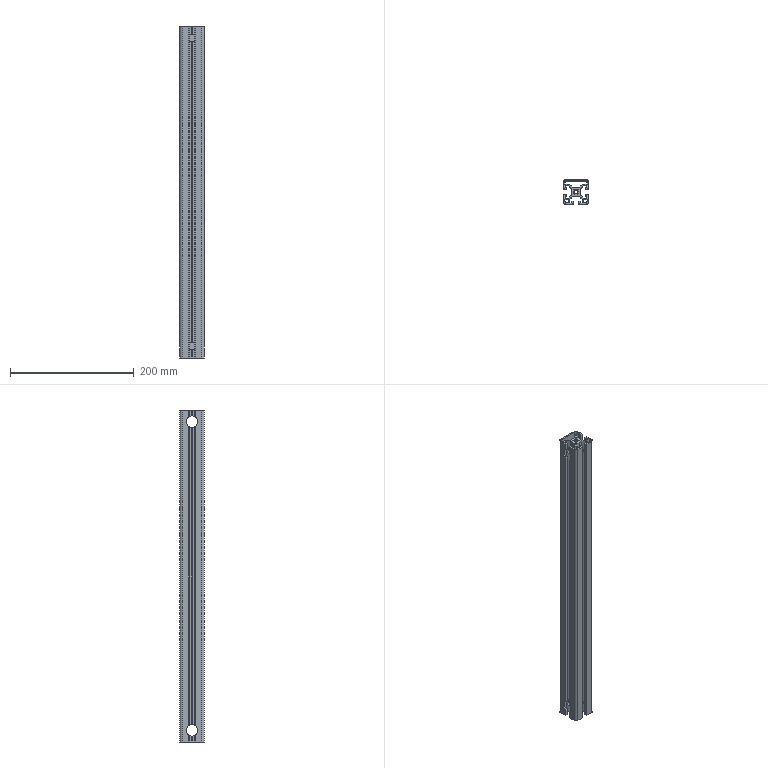Part | SolidWorks | features BaseBody 1, HoleWzd 1, MoveFace 1 | 1 solid | 242 faces | box 40 x 40 x 536 mm | volume 308966 mm3 | plane 187 | cylinder 55 | commonest cylinder face diameters 6.8 x15 2 x14 19 x12 1 x6 5 x4 9 x4